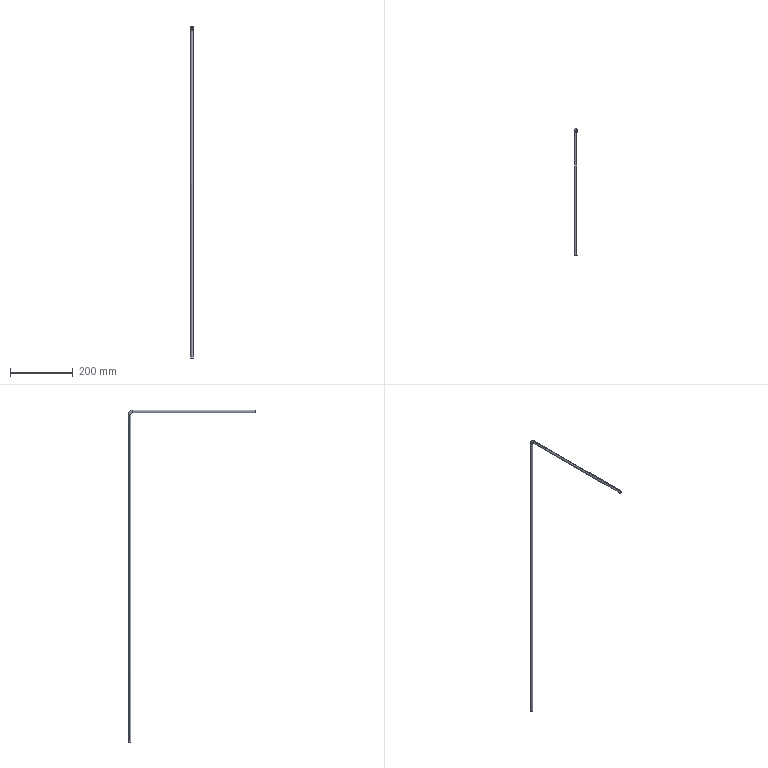Part | SolidWorks | features Sweep 1 | 1 solid | 14 faces | box 8 x 404 x 1054 mm | volume 31793 mm3 | cylinder 8 | torus 4 | plane 2 | commonest cylinder face diameters 6 x4 8 x4
STEP:
#1=CARTESIAN_POINT('',(0.,390.,-3.));
#2=VERTEX_POINT('',#1);
#3=CARTESIAN_POINT('',(0.,390.,3.));
#4=VERTEX_POINT('',#3);
#5=CARTESIAN_POINT('',(0.,390.,0.));
#6=DIRECTION('',(0.,-1.,0.));
#7=DIRECTION('',(0.,0.,1.));
#8=AXIS2_PLACEMENT_3D('',#5,#6,#7);
#9=CIRCLE('',#8,3.);
#10=EDGE_CURVE('',#2,#4,#9,.T.);
#11=ORIENTED_EDGE('',*,*,#10,.T.);
#12=CARTESIAN_POINT('',(0.,403.,-10.));
#13=VERTEX_POINT('',#12);
#14=CARTESIAN_POINT('',(0.,390.,-10.));
#15=DIRECTION('',(-1.,0.,0.));
#16=DIRECTION('',(0.,0.,1.));
#17=AXIS2_PLACEMENT_3D('',#14,#15,#16);
#18=CIRCLE('',#17,13.);
#19=EDGE_CURVE('',#4,#13,#18,.T.);
#20=ORIENTED_EDGE('',*,*,#19,.T.);
#21=CARTESIAN_POINT('',(3.,400.,-10.));
#22=VERTEX_POINT('',#21);
#23=CARTESIAN_POINT('',(0.,400.,-10.));
#24=DIRECTION('',(0.,0.,1.));
#25=DIRECTION('',(0.,1.,0.));
#26=AXIS2_PLACEMENT_3D('',#23,#24,#25);
#27=CIRCLE('',#26,3.);
#28=EDGE_CURVE('',#22,#13,#27,.T.);
#29=ORIENTED_EDGE('',*,*,#28,.F.);
#30=CARTESIAN_POINT('',(0.,397.,-10.));
#31=VERTEX_POINT('',#30);
#32=CARTESIAN_POINT('',(0.,400.,-10.));
#33=DIRECTION('',(0.,0.,1.));
#34=DIRECTION('',(0.,1.,0.));
#35=AXIS2_PLACEMENT_3D('',#32,#33,#34);
#36=CIRCLE('',#35,3.);
#37=EDGE_CURVE('',#31,#22,#36,.T.);
#38=ORIENTED_EDGE('',*,*,#37,.F.);
#39=CARTESIAN_POINT('',(0.,390.,-10.));
#40=DIRECTION('',(-1.,0.,0.));
#41=DIRECTION('',(0.,0.,1.));
#42=AXIS2_PLACEMENT_3D('',#39,#40,#41);
#43=CIRCLE('',#42,7.);
#44=EDGE_CURVE('',#2,#31,#43,.T.);
#45=ORIENTED_EDGE('',*,*,#44,.F.);
#46=EDGE_LOOP('',(#11,#20,#29,#38,#45));
#47=FACE_OUTER_BOUND('',#46,.T.);
#48=CARTESIAN_POINT('',(0.,390.,-10.));
#49=DIRECTION('',(-1.,0.,0.));
#50=DIRECTION('',(0.,0.,1.));
#51=AXIS2_PLACEMENT_3D('',#48,#49,#50);
#52=TOROIDAL_SURFACE('',#51,10.,3.);
#53=ADVANCED_FACE('',(#47),#52,.F.);
#54=CARTESIAN_POINT('',(0.,390.,-4.));
#55=VERTEX_POINT('',#54);
#56=CARTESIAN_POINT('',(0.,390.,4.));
#57=VERTEX_POINT('',#56);
#58=CARTESIAN_POINT('',(0.,390.,0.));
#59=DIRECTION('',(0.,1.,0.));
#60=DIRECTION('',(0.,0.,1.));
#61=AXIS2_PLACEMENT_3D('',#58,#59,#60);
#62=CIRCLE('',#61,4.);
#63=EDGE_CURVE('',#55,#57,#62,.T.);
#64=ORIENTED_EDGE('',*,*,#63,.T.);
#65=CARTESIAN_POINT('',(0.,404.,-10.));
#66=VERTEX_POINT('',#65);
#67=CARTESIAN_POINT('',(0.,390.,-10.));
#68=DIRECTION('',(-1.,0.,0.));
#69=DIRECTION('',(0.,0.,1.));
#70=AXIS2_PLACEMENT_3D('',#67,#68,#69);
#71=CIRCLE('',#70,14.);
#72=EDGE_CURVE('',#57,#66,#71,.T.);
#73=ORIENTED_EDGE('',*,*,#72,.T.);
#74=CARTESIAN_POINT('',(-4.,400.,-10.));
#75=VERTEX_POINT('',#74);
#76=CARTESIAN_POINT('',(0.,400.,-10.));
#77=DIRECTION('',(0.,0.,-1.));
#78=DIRECTION('',(0.,1.,0.));
#79=AXIS2_PLACEMENT_3D('',#76,#77,#78);
#80=CIRCLE('',#79,4.);
#81=EDGE_CURVE('',#75,#66,#80,.T.);
#82=ORIENTED_EDGE('',*,*,#81,.F.);
#83=CARTESIAN_POINT('',(0.,396.,-10.));
#84=VERTEX_POINT('',#83);
#85=CARTESIAN_POINT('',(0.,400.,-10.));
#86=DIRECTION('',(0.,0.,-1.));
#87=DIRECTION('',(0.,1.,0.));
#88=AXIS2_PLACEMENT_3D('',#85,#86,#87);
#89=CIRCLE('',#88,4.);
#90=EDGE_CURVE('',#84,#75,#89,.T.);
#91=ORIENTED_EDGE('',*,*,#90,.F.);
#92=CARTESIAN_POINT('',(0.,390.,-10.));
#93=DIRECTION('',(-1.,0.,0.));
#94=DIRECTION('',(0.,0.,1.));
#95=AXIS2_PLACEMENT_3D('',#92,#93,#94);
#96=CIRCLE('',#95,6.);
#97=EDGE_CURVE('',#55,#84,#96,.T.);
#98=ORIENTED_EDGE('',*,*,#97,.F.);
#99=EDGE_LOOP('',(#64,#73,#82,#91,#98));
#100=FACE_OUTER_BOUND('',#99,.T.);
#101=CARTESIAN_POINT('',(0.,390.,-10.));
#102=DIRECTION('',(-1.,0.,0.));
#103=DIRECTION('',(0.,0.,1.));
#104=AXIS2_PLACEMENT_3D('',#101,#102,#103);
#105=TOROIDAL_SURFACE('',#104,10.,4.);
#106=ADVANCED_FACE('',(#100),#105,.T.);
#107=CARTESIAN_POINT('',(-3.,400.,-10.));
#108=VERTEX_POINT('',#107);
#109=CARTESIAN_POINT('',(0.,400.,-10.));
#110=DIRECTION('',(0.,0.,1.));
#111=DIRECTION('',(0.,1.,0.));
#112=AXIS2_PLACEMENT_3D('',#109,#110,#111);
#113=CIRCLE('',#112,3.);
#114=EDGE_CURVE('',#108,#31,#113,.T.);
#115=ORIENTED_EDGE('',*,*,#114,.T.);
#116=ORIENTED_EDGE('',*,*,#37,.T.);
#117=CARTESIAN_POINT('',(3.,400.,-1050.));
#118=VERTEX_POINT('',#117);
#119=CARTESIAN_POINT('',(3.,400.,-10.));
#120=DIRECTION('',(0.,0.,-1.));
#121=VECTOR('',#120,1000.);
#122=LINE('',#119,#121);
#123=EDGE_CURVE('',#22,#118,#122,.T.);
#124=ORIENTED_EDGE('',*,*,#123,.T.);
#125=CARTESIAN_POINT('',(-3.,400.,-1050.));
#126=VERTEX_POINT('',#125);
#127=CARTESIAN_POINT('',(0.,400.,-1050.));
#128=DIRECTION('',(0.,0.,1.));
#129=DIRECTION('',(0.,1.,0.));
#130=AXIS2_PLACEMENT_3D('',#127,#128,#129);
#131=CIRCLE('',#130,3.);
#132=EDGE_CURVE('',#126,#118,#131,.T.);
#133=ORIENTED_EDGE('',*,*,#132,.F.);
#134=CARTESIAN_POINT('',(-3.,400.,-10.));
#135=DIRECTION('',(0.,0.,-1.));
#136=VECTOR('',#135,1000.);
#137=LINE('',#134,#136);
#138=EDGE_CURVE('',#108,#126,#137,.T.);
#139=ORIENTED_EDGE('',*,*,#138,.F.);
#140=EDGE_LOOP('',(#115,#116,#124,#133,#139));
#141=FACE_OUTER_BOUND('',#140,.T.);
#142=CARTESIAN_POINT('',(0.,400.,-10.));
#143=DIRECTION('',(0.,0.,-1.));
#144=DIRECTION('',(-1.,0.,0.));
#145=AXIS2_PLACEMENT_3D('',#142,#143,#144);
#146=CYLINDRICAL_SURFACE('',#145,3.);
#147=ADVANCED_FACE('',(#141),#146,.F.);
#148=CARTESIAN_POINT('',(0.,0.,3.));
#149=VERTEX_POINT('',#148);
#150=CARTESIAN_POINT('',(0.,0.,-3.));
#151=VERTEX_POINT('',#150);
#152=CARTESIAN_POINT('',(0.,0.,0.));
#153=DIRECTION('',(0.,-1.,0.));
#154=DIRECTION('',(0.,0.,1.));
#155=AXIS2_PLACEMENT_3D('',#152,#153,#154);
#156=CIRCLE('',#155,3.);
#157=EDGE_CURVE('',#149,#151,#156,.T.);
#158=ORIENTED_EDGE('',*,*,#157,.T.);
#159=CARTESIAN_POINT('',(0.,0.,-3.));
#160=DIRECTION('',(0.,1.,0.));
#161=VECTOR('',#160,1000.);
#162=LINE('',#159,#161);
#163=EDGE_CURVE('',#151,#2,#162,.T.);
#164=ORIENTED_EDGE('',*,*,#163,.T.);
#165=CARTESIAN_POINT('',(0.,390.,0.));
#166=DIRECTION('',(0.,-1.,0.));
#167=DIRECTION('',(0.,0.,1.));
#168=AXIS2_PLACEMENT_3D('',#165,#166,#167);
#169=CIRCLE('',#168,3.);
#170=EDGE_CURVE('',#4,#2,#169,.T.);
#171=ORIENTED_EDGE('',*,*,#170,.F.);
#172=CARTESIAN_POINT('',(0.,0.,3.));
#173=DIRECTION('',(0.,1.,0.));
#174=VECTOR('',#173,1000.);
#175=LINE('',#172,#174);
#176=EDGE_CURVE('',#149,#4,#175,.T.);
#177=ORIENTED_EDGE('',*,*,#176,.F.);
#178=EDGE_LOOP('',(#158,#164,#171,#177));
#179=FACE_OUTER_BOUND('',#178,.T.);
#180=CARTESIAN_POINT('',(0.,0.,0.));
#181=DIRECTION('',(0.,1.,0.));
#182=DIRECTION('',(0.,0.,1.));
#183=AXIS2_PLACEMENT_3D('',#180,#181,#182);
#184=CYLINDRICAL_SURFACE('',#183,3.);
#185=ADVANCED_FACE('',(#179),#184,.F.);
#186=ORIENTED_EDGE('',*,*,#81,.T.);
#187=CARTESIAN_POINT('',(4.,400.,-10.));
#188=VERTEX_POINT('',#187);
#189=CARTESIAN_POINT('',(0.,400.,-10.));
#190=DIRECTION('',(0.,0.,-1.));
#191=DIRECTION('',(0.,1.,0.));
#192=AXIS2_PLACEMENT_3D('',#189,#190,#191);
#193=CIRCLE('',#192,4.);
#194=EDGE_CURVE('',#66,#188,#193,.T.);
#195=ORIENTED_EDGE('',*,*,#194,.T.);
#196=CARTESIAN_POINT('',(4.,400.,-1050.));
#197=VERTEX_POINT('',#196);
#198=CARTESIAN_POINT('',(4.,400.,-10.));
#199=DIRECTION('',(0.,0.,-1.));
#200=VECTOR('',#199,1000.);
#201=LINE('',#198,#200);
#202=EDGE_CURVE('',#188,#197,#201,.T.);
#203=ORIENTED_EDGE('',*,*,#202,.T.);
#204=CARTESIAN_POINT('',(-4.,400.,-1050.));
#205=VERTEX_POINT('',#204);
#206=CARTESIAN_POINT('',(0.,400.,-1050.));
#207=DIRECTION('',(0.,0.,-1.));
#208=DIRECTION('',(0.,1.,0.));
#209=AXIS2_PLACEMENT_3D('',#206,#207,#208);
#210=CIRCLE('',#209,4.);
#211=EDGE_CURVE('',#205,#197,#210,.T.);
#212=ORIENTED_EDGE('',*,*,#211,.F.);
#213=CARTESIAN_POINT('',(-4.,400.,-10.));
#214=DIRECTION('',(0.,0.,-1.));
#215=VECTOR('',#214,1000.);
#216=LINE('',#213,#215);
#217=EDGE_CURVE('',#75,#205,#216,.T.);
#218=ORIENTED_EDGE('',*,*,#217,.F.);
#219=EDGE_LOOP('',(#186,#195,#203,#212,#218));
#220=FACE_OUTER_BOUND('',#219,.T.);
#221=CARTESIAN_POINT('',(0.,400.,-10.));
#222=DIRECTION('',(0.,0.,-1.));
#223=DIRECTION('',(-1.,0.,0.));
#224=AXIS2_PLACEMENT_3D('',#221,#222,#223);
#225=CYLINDRICAL_SURFACE('',#224,4.);
#226=ADVANCED_FACE('',(#220),#225,.T.);
#227=CARTESIAN_POINT('',(0.,0.,4.));
#228=VERTEX_POINT('',#227);
#229=CARTESIAN_POINT('',(0.,0.,-4.));
#230=VERTEX_POINT('',#229);
#231=CARTESIAN_POINT('',(0.,0.,0.));
#232=DIRECTION('',(0.,1.,0.));
#233=DIRECTION('',(0.,0.,1.));
#234=AXIS2_PLACEMENT_3D('',#231,#232,#233);
#235=CIRCLE('',#234,4.);
#236=EDGE_CURVE('',#228,#230,#235,.T.);
#237=ORIENTED_EDGE('',*,*,#236,.T.);
#238=CARTESIAN_POINT('',(0.,0.,-4.));
#239=DIRECTION('',(0.,1.,0.));
#240=VECTOR('',#239,1000.);
#241=LINE('',#238,#240);
#242=EDGE_CURVE('',#230,#55,#241,.T.);
#243=ORIENTED_EDGE('',*,*,#242,.T.);
#244=CARTESIAN_POINT('',(0.,390.,0.));
#245=DIRECTION('',(0.,1.,0.));
#246=DIRECTION('',(0.,0.,1.));
#247=AXIS2_PLACEMENT_3D('',#244,#245,#246);
#248=CIRCLE('',#247,4.);
#249=EDGE_CURVE('',#57,#55,#248,.T.);
#250=ORIENTED_EDGE('',*,*,#249,.F.);
#251=CARTESIAN_POINT('',(0.,0.,4.));
#252=DIRECTION('',(0.,1.,0.));
#253=VECTOR('',#252,1000.);
#254=LINE('',#251,#253);
#255=EDGE_CURVE('',#228,#57,#254,.T.);
#256=ORIENTED_EDGE('',*,*,#255,.F.);
#257=EDGE_LOOP('',(#237,#243,#250,#256));
#258=FACE_OUTER_BOUND('',#257,.T.);
#259=CARTESIAN_POINT('',(0.,0.,0.));
#260=DIRECTION('',(0.,1.,0.));
#261=DIRECTION('',(0.,0.,1.));
#262=AXIS2_PLACEMENT_3D('',#259,#260,#261);
#263=CYLINDRICAL_SURFACE('',#262,4.);
#264=ADVANCED_FACE('',(#258),#263,.T.);
#265=ORIENTED_EDGE('',*,*,#123,.F.);
#266=ORIENTED_EDGE('',*,*,#28,.T.);
#267=CARTESIAN_POINT('',(0.,400.,-10.));
#268=DIRECTION('',(0.,0.,1.));
#269=DIRECTION('',(0.,1.,0.));
#270=AXIS2_PLACEMENT_3D('',#267,#268,#269);
#271=CIRCLE('',#270,3.);
#272=EDGE_CURVE('',#13,#108,#271,.T.);
#273=ORIENTED_EDGE('',*,*,#272,.T.);
#274=ORIENTED_EDGE('',*,*,#138,.T.);
#275=CARTESIAN_POINT('',(0.,400.,-1050.));
#276=DIRECTION('',(0.,0.,1.));
#277=DIRECTION('',(0.,1.,0.));
#278=AXIS2_PLACEMENT_3D('',#275,#276,#277);
#279=CIRCLE('',#278,3.);
#280=EDGE_CURVE('',#118,#126,#279,.T.);
#281=ORIENTED_EDGE('',*,*,#280,.F.);
#282=EDGE_LOOP('',(#265,#266,#273,#274,#281));
#283=FACE_OUTER_BOUND('',#282,.T.);
#284=CARTESIAN_POINT('',(0.,400.,-10.));
#285=DIRECTION('',(0.,0.,-1.));
#286=DIRECTION('',(-1.,0.,0.));
#287=AXIS2_PLACEMENT_3D('',#284,#285,#286);
#288=CYLINDRICAL_SURFACE('',#287,3.);
#289=ADVANCED_FACE('',(#283),#288,.F.);
#290=ORIENTED_EDGE('',*,*,#19,.F.);
#291=ORIENTED_EDGE('',*,*,#170,.T.);
#292=ORIENTED_EDGE('',*,*,#44,.T.);
#293=ORIENTED_EDGE('',*,*,#114,.F.);
#294=ORIENTED_EDGE('',*,*,#272,.F.);
#295=EDGE_LOOP('',(#290,#291,#292,#293,#294));
#296=FACE_OUTER_BOUND('',#295,.T.);
#297=CARTESIAN_POINT('',(0.,390.,-10.));
#298=DIRECTION('',(-1.,0.,0.));
#299=DIRECTION('',(0.,0.,1.));
#300=AXIS2_PLACEMENT_3D('',#297,#298,#299);
#301=TOROIDAL_SURFACE('',#300,10.,3.);
#302=ADVANCED_FACE('',(#296),#301,.F.);
#303=ORIENTED_EDGE('',*,*,#163,.F.);
#304=CARTESIAN_POINT('',(0.,0.,0.));
#305=DIRECTION('',(0.,-1.,0.));
#306=DIRECTION('',(0.,0.,1.));
#307=AXIS2_PLACEMENT_3D('',#304,#305,#306);
#308=CIRCLE('',#307,3.);
#309=EDGE_CURVE('',#151,#149,#308,.T.);
#310=ORIENTED_EDGE('',*,*,#309,.T.);
#311=ORIENTED_EDGE('',*,*,#176,.T.);
#312=ORIENTED_EDGE('',*,*,#10,.F.);
#313=EDGE_LOOP('',(#303,#310,#311,#312));
#314=FACE_OUTER_BOUND('',#313,.T.);
#315=CARTESIAN_POINT('',(0.,0.,0.));
#316=DIRECTION('',(0.,1.,0.));
#317=DIRECTION('',(0.,0.,1.));
#318=AXIS2_PLACEMENT_3D('',#315,#316,#317);
#319=CYLINDRICAL_SURFACE('',#318,3.);
#320=ADVANCED_FACE('',(#314),#319,.F.);
#321=ORIENTED_EDGE('',*,*,#132,.T.);
#322=ORIENTED_EDGE('',*,*,#280,.T.);
#323=EDGE_LOOP('',(#321,#322));
#324=FACE_BOUND('',#323,.T.);
#325=ORIENTED_EDGE('',*,*,#211,.T.);
#326=CARTESIAN_POINT('',(0.,400.,-1050.));
#327=DIRECTION('',(0.,0.,-1.));
#328=DIRECTION('',(0.,1.,0.));
#329=AXIS2_PLACEMENT_3D('',#326,#327,#328);
#330=CIRCLE('',#329,4.);
#331=EDGE_CURVE('',#197,#205,#330,.T.);
#332=ORIENTED_EDGE('',*,*,#331,.T.);
#333=EDGE_LOOP('',(#325,#332));
#334=FACE_OUTER_BOUND('',#333,.T.);
#335=CARTESIAN_POINT('',(0.,400.,-1050.));
#336=DIRECTION('',(0.,0.,-1.));
#337=DIRECTION('',(0.,1.,0.));
#338=AXIS2_PLACEMENT_3D('',#335,#336,#337);
#339=PLANE('',#338);
#340=ADVANCED_FACE('',(#324,#334),#339,.T.);
#341=ORIENTED_EDGE('',*,*,#157,.F.);
#342=ORIENTED_EDGE('',*,*,#309,.F.);
#343=EDGE_LOOP('',(#341,#342));
#344=FACE_BOUND('',#343,.T.);
#345=ORIENTED_EDGE('',*,*,#236,.F.);
#346=CARTESIAN_POINT('',(0.,0.,0.));
#347=DIRECTION('',(0.,1.,0.));
#348=DIRECTION('',(0.,0.,1.));
#349=AXIS2_PLACEMENT_3D('',#346,#347,#348);
#350=CIRCLE('',#349,4.);
#351=EDGE_CURVE('',#230,#228,#350,.T.);
#352=ORIENTED_EDGE('',*,*,#351,.F.);
#353=EDGE_LOOP('',(#345,#352));
#354=FACE_OUTER_BOUND('',#353,.T.);
#355=CARTESIAN_POINT('',(0.,0.,0.));
#356=DIRECTION('',(0.,1.,0.));
#357=DIRECTION('',(0.,0.,1.));
#358=AXIS2_PLACEMENT_3D('',#355,#356,#357);
#359=PLANE('',#358);
#360=ADVANCED_FACE('',(#344,#354),#359,.F.);
#361=ORIENTED_EDGE('',*,*,#202,.F.);
#362=CARTESIAN_POINT('',(0.,400.,-10.));
#363=DIRECTION('',(0.,0.,-1.));
#364=DIRECTION('',(0.,1.,0.));
#365=AXIS2_PLACEMENT_3D('',#362,#363,#364);
#366=CIRCLE('',#365,4.);
#367=EDGE_CURVE('',#188,#84,#366,.T.);
#368=ORIENTED_EDGE('',*,*,#367,.T.);
#369=ORIENTED_EDGE('',*,*,#90,.T.);
#370=ORIENTED_EDGE('',*,*,#217,.T.);
#371=ORIENTED_EDGE('',*,*,#331,.F.);
#372=EDGE_LOOP('',(#361,#368,#369,#370,#371));
#373=FACE_OUTER_BOUND('',#372,.T.);
#374=CARTESIAN_POINT('',(0.,400.,-10.));
#375=DIRECTION('',(0.,0.,-1.));
#376=DIRECTION('',(-1.,0.,0.));
#377=AXIS2_PLACEMENT_3D('',#374,#375,#376);
#378=CYLINDRICAL_SURFACE('',#377,4.);
#379=ADVANCED_FACE('',(#373),#378,.T.);
#380=ORIENTED_EDGE('',*,*,#72,.F.);
#381=ORIENTED_EDGE('',*,*,#249,.T.);
#382=ORIENTED_EDGE('',*,*,#97,.T.);
#383=ORIENTED_EDGE('',*,*,#367,.F.);
#384=ORIENTED_EDGE('',*,*,#194,.F.);
#385=EDGE_LOOP('',(#380,#381,#382,#383,#384));
#386=FACE_OUTER_BOUND('',#385,.T.);
#387=CARTESIAN_POINT('',(0.,390.,-10.));
#388=DIRECTION('',(-1.,0.,0.));
#389=DIRECTION('',(0.,0.,1.));
#390=AXIS2_PLACEMENT_3D('',#387,#388,#389);
#391=TOROIDAL_SURFACE('',#390,10.,4.);
#392=ADVANCED_FACE('',(#386),#391,.T.);
#393=ORIENTED_EDGE('',*,*,#242,.F.);
#394=ORIENTED_EDGE('',*,*,#351,.T.);
#395=ORIENTED_EDGE('',*,*,#255,.T.);
#396=ORIENTED_EDGE('',*,*,#63,.F.);
#397=EDGE_LOOP('',(#393,#394,#395,#396));
#398=FACE_OUTER_BOUND('',#397,.T.);
#399=CARTESIAN_POINT('',(0.,0.,0.));
#400=DIRECTION('',(0.,1.,0.));
#401=DIRECTION('',(0.,0.,1.));
#402=AXIS2_PLACEMENT_3D('',#399,#400,#401);
#403=CYLINDRICAL_SURFACE('',#402,4.);
#404=ADVANCED_FACE('',(#398),#403,.T.);
#405=CLOSED_SHELL('',(#53,#106,#147,#185,#226,#264,#289,#302,#320,#340,#360,#379,#392,#404));
#406=MANIFOLD_SOLID_BREP('',#405);
#407=CARTESIAN_POINT('',(0.,0.,0.));
#408=DIRECTION('',(0.,0.,1.));
#409=DIRECTION('',(1.,0.,0.));
#410=AXIS2_PLACEMENT_3D('',#407,#408,#409);
#411=(LENGTH_UNIT()NAMED_UNIT(*)SI_UNIT(.MILLI.,.METRE.));
#412=UNCERTAINTY_MEASURE_WITH_UNIT(LENGTH_MEASURE(0.00001),#411,'','');
#413=(NAMED_UNIT(*)PLANE_ANGLE_UNIT()SI_UNIT($,.RADIAN.));
#414=(NAMED_UNIT(*)SI_UNIT($,.STERADIAN.)SOLID_ANGLE_UNIT());
#415=(GEOMETRIC_REPRESENTATION_CONTEXT(3)GLOBAL_UNCERTAINTY_ASSIGNED_CONTEXT((#412))GLOBAL_UNIT_ASSIGNED_CONTEXT((#411,#413,#414))REPRESENTATION_CONTEXT('',''));
#416=ADVANCED_BREP_SHAPE_REPRESENTATION('',(#406,#410),#415);